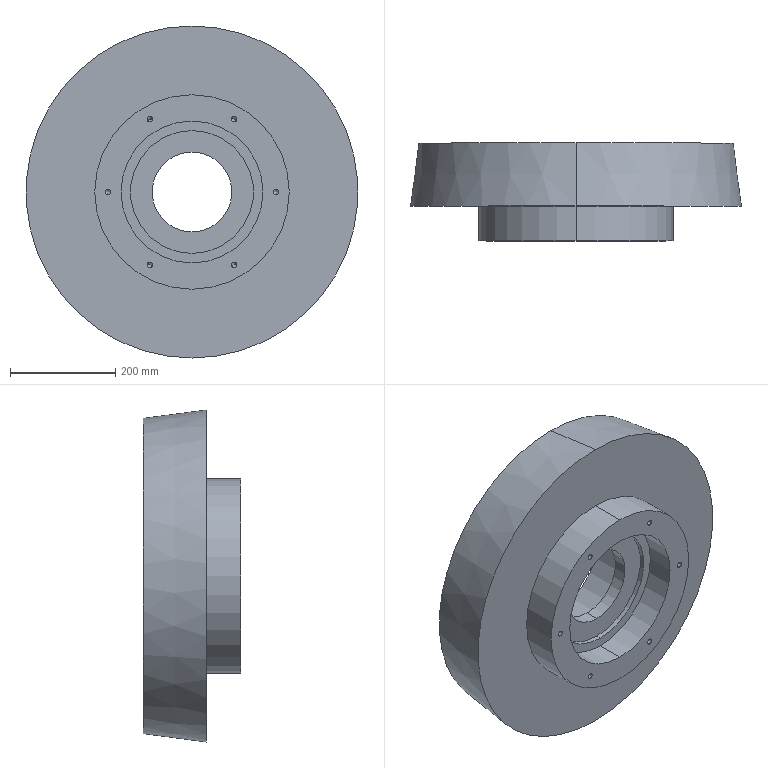Part | SolidWorks | features 3DProfileFeature 2, CirPattern 2, HoleWzd 2, Revolution 1 | 1 solid | 69 faces | box 631.597 x 186 x 631.597 mm | volume 33435702 mm3 | cylinder 36 | cone 26 | plane 7 | commonest cylinder face diameters 10.716 x24 234 x4 270 x4 152 x2 370 x2